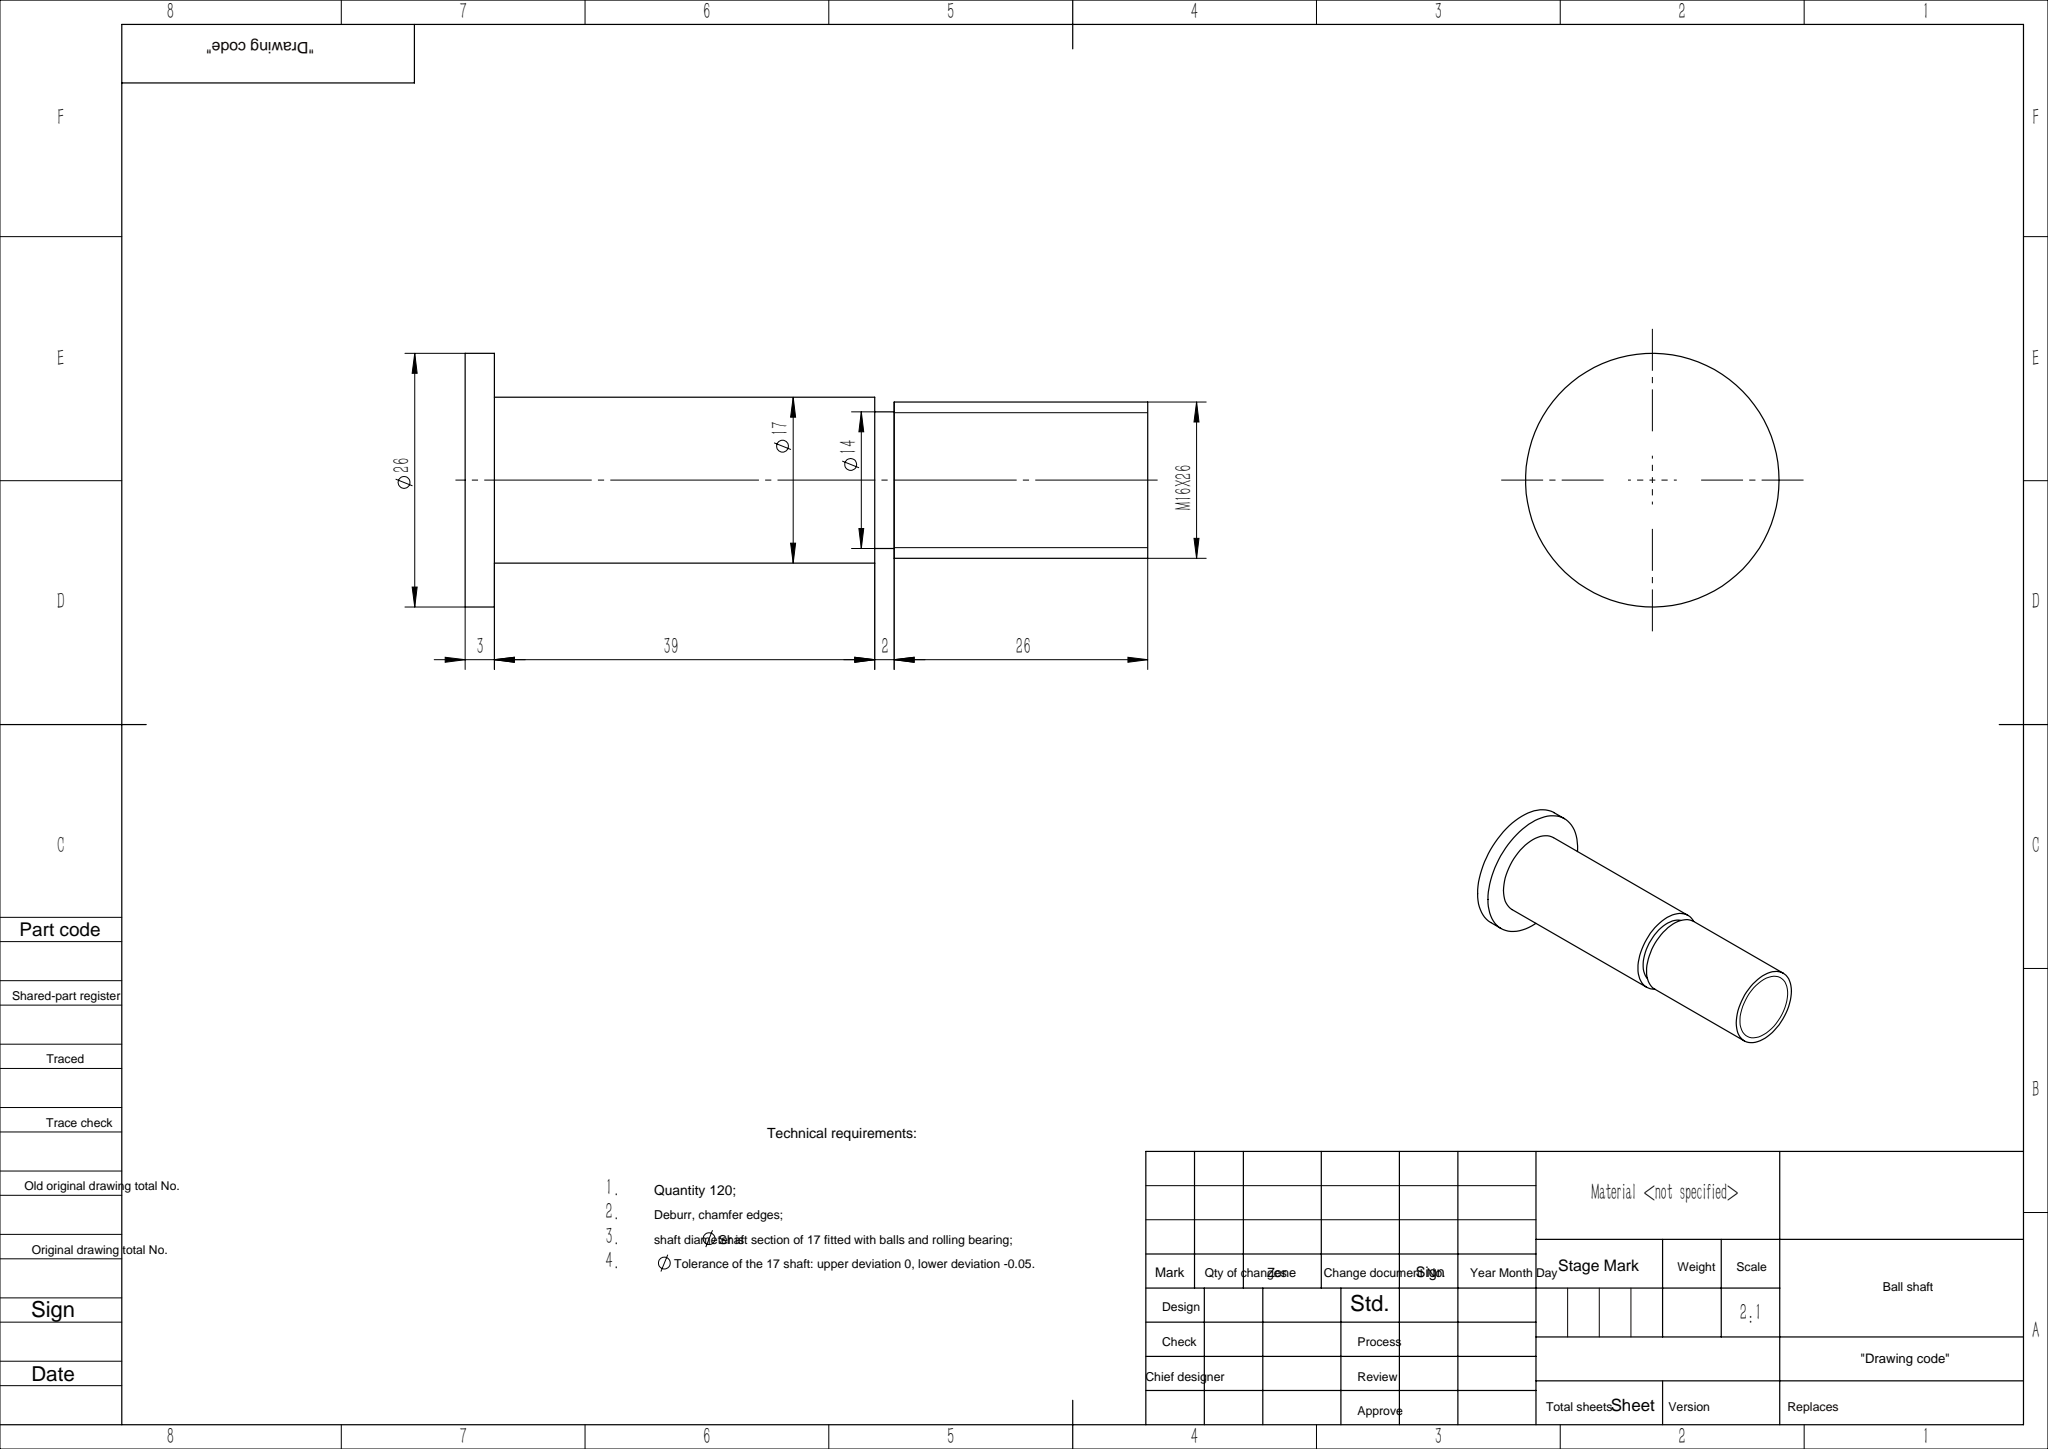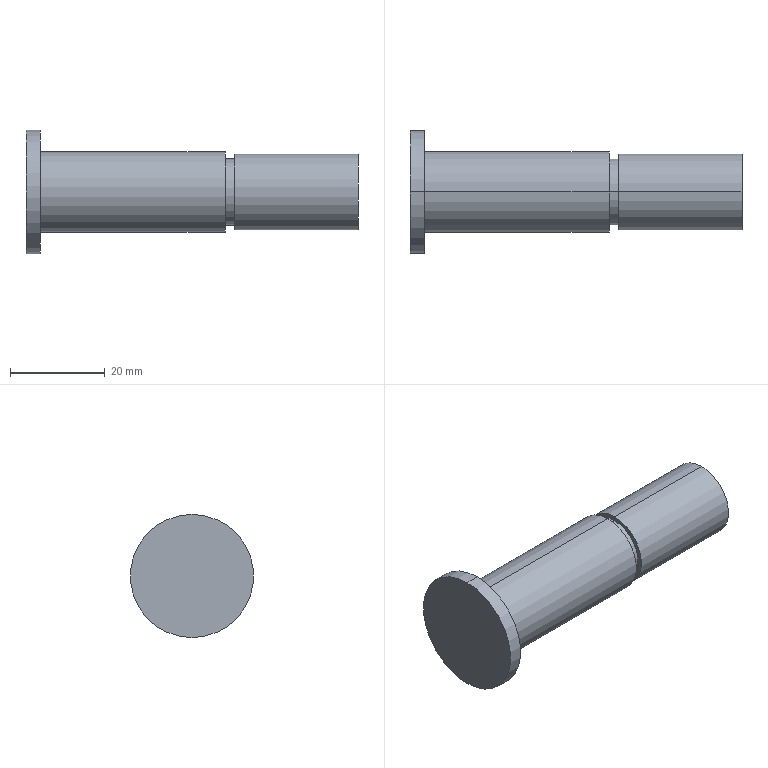Part | SolidWorks | features ICE 2, Revolution 1 | 1 solid | 13 faces | box 70 x 26 x 26 mm | volume 15980 mm3 | cylinder 8 | plane 5 | commonest cylinder face diameters 14 x2 16 x2 17 x2 26 x2
STEP:
#1=CARTESIAN_POINT('',(44.,0.,-8.));
#2=VERTEX_POINT('',#1);
#3=CARTESIAN_POINT('',(44.,0.,8.));
#4=VERTEX_POINT('',#3);
#5=CARTESIAN_POINT('',(44.,0.,0.));
#6=DIRECTION('',(1.,0.,0.));
#7=DIRECTION('',(0.,0.,-1.));
#8=AXIS2_PLACEMENT_3D('',#5,#6,#7);
#9=CIRCLE('',#8,8.);
#10=EDGE_CURVE('',#2,#4,#9,.T.);
#11=ORIENTED_EDGE('',*,*,#10,.T.);
#12=CARTESIAN_POINT('',(70.,0.,8.));
#13=VERTEX_POINT('',#12);
#14=CARTESIAN_POINT('',(42.,0.,8.));
#15=DIRECTION('',(1.,0.,0.));
#16=VECTOR('',#15,1000.);
#17=LINE('',#14,#16);
#18=EDGE_CURVE('',#4,#13,#17,.T.);
#19=ORIENTED_EDGE('',*,*,#18,.T.);
#20=CARTESIAN_POINT('',(70.,0.,-8.));
#21=VERTEX_POINT('',#20);
#22=CARTESIAN_POINT('',(70.,0.,0.));
#23=DIRECTION('',(1.,0.,0.));
#24=DIRECTION('',(0.,0.,-1.));
#25=AXIS2_PLACEMENT_3D('',#22,#23,#24);
#26=CIRCLE('',#25,8.);
#27=EDGE_CURVE('',#21,#13,#26,.T.);
#28=ORIENTED_EDGE('',*,*,#27,.F.);
#29=CARTESIAN_POINT('',(42.,0.,-8.));
#30=DIRECTION('',(1.,0.,0.));
#31=VECTOR('',#30,1000.);
#32=LINE('',#29,#31);
#33=EDGE_CURVE('',#2,#21,#32,.T.);
#34=ORIENTED_EDGE('',*,*,#33,.F.);
#35=EDGE_LOOP('',(#11,#19,#28,#34));
#36=FACE_OUTER_BOUND('',#35,.T.);
#37=CARTESIAN_POINT('',(42.,0.,0.));
#38=DIRECTION('',(1.,0.,0.));
#39=DIRECTION('',(0.,0.,-1.));
#40=AXIS2_PLACEMENT_3D('',#37,#38,#39);
#41=CYLINDRICAL_SURFACE('',#40,8.);
#42=ADVANCED_FACE('',(#36),#41,.T.);
#43=CARTESIAN_POINT('',(44.,0.,-7.));
#44=VERTEX_POINT('',#43);
#45=CARTESIAN_POINT('',(44.,0.,7.));
#46=VERTEX_POINT('',#45);
#47=CARTESIAN_POINT('',(44.,0.,0.));
#48=DIRECTION('',(1.,0.,0.));
#49=DIRECTION('',(0.,0.,-1.));
#50=AXIS2_PLACEMENT_3D('',#47,#48,#49);
#51=CIRCLE('',#50,7.);
#52=EDGE_CURVE('',#44,#46,#51,.T.);
#53=ORIENTED_EDGE('',*,*,#52,.F.);
#54=CARTESIAN_POINT('',(42.,0.,-7.));
#55=VERTEX_POINT('',#54);
#56=CARTESIAN_POINT('',(44.,0.,-7.));
#57=DIRECTION('',(-1.,0.,0.));
#58=VECTOR('',#57,1000.);
#59=LINE('',#56,#58);
#60=EDGE_CURVE('',#44,#55,#59,.T.);
#61=ORIENTED_EDGE('',*,*,#60,.T.);
#62=CARTESIAN_POINT('',(42.,0.,7.));
#63=VERTEX_POINT('',#62);
#64=CARTESIAN_POINT('',(42.,0.,0.));
#65=DIRECTION('',(1.,0.,0.));
#66=DIRECTION('',(0.,0.,-1.));
#67=AXIS2_PLACEMENT_3D('',#64,#65,#66);
#68=CIRCLE('',#67,7.);
#69=EDGE_CURVE('',#55,#63,#68,.T.);
#70=ORIENTED_EDGE('',*,*,#69,.T.);
#71=CARTESIAN_POINT('',(44.,0.,7.));
#72=DIRECTION('',(-1.,0.,0.));
#73=VECTOR('',#72,1000.);
#74=LINE('',#71,#73);
#75=EDGE_CURVE('',#46,#63,#74,.T.);
#76=ORIENTED_EDGE('',*,*,#75,.F.);
#77=EDGE_LOOP('',(#53,#61,#70,#76));
#78=FACE_OUTER_BOUND('',#77,.T.);
#79=CARTESIAN_POINT('',(44.,0.,0.));
#80=DIRECTION('',(-1.,0.,0.));
#81=DIRECTION('',(0.,0.,1.));
#82=AXIS2_PLACEMENT_3D('',#79,#80,#81);
#83=CYLINDRICAL_SURFACE('',#82,7.);
#84=ADVANCED_FACE('',(#78),#83,.T.);
#85=CARTESIAN_POINT('',(3.,0.,13.));
#86=VERTEX_POINT('',#85);
#87=CARTESIAN_POINT('',(3.,0.,-13.));
#88=VERTEX_POINT('',#87);
#89=CARTESIAN_POINT('',(3.,0.,0.));
#90=DIRECTION('',(-1.,0.,0.));
#91=DIRECTION('',(0.,0.,1.));
#92=AXIS2_PLACEMENT_3D('',#89,#90,#91);
#93=CIRCLE('',#92,13.);
#94=EDGE_CURVE('',#86,#88,#93,.T.);
#95=ORIENTED_EDGE('',*,*,#94,.T.);
#96=CARTESIAN_POINT('',(0.,0.,-13.));
#97=VERTEX_POINT('',#96);
#98=CARTESIAN_POINT('',(0.,0.,-13.));
#99=DIRECTION('',(-1.,0.,0.));
#100=VECTOR('',#99,1000.);
#101=LINE('',#98,#100);
#102=EDGE_CURVE('',#88,#97,#101,.T.);
#103=ORIENTED_EDGE('',*,*,#102,.T.);
#104=CARTESIAN_POINT('',(0.,0.,13.));
#105=VERTEX_POINT('',#104);
#106=CARTESIAN_POINT('',(0.,0.,0.));
#107=DIRECTION('',(-1.,0.,0.));
#108=DIRECTION('',(0.,0.,1.));
#109=AXIS2_PLACEMENT_3D('',#106,#107,#108);
#110=CIRCLE('',#109,13.);
#111=EDGE_CURVE('',#105,#97,#110,.T.);
#112=ORIENTED_EDGE('',*,*,#111,.F.);
#113=CARTESIAN_POINT('',(0.,0.,13.));
#114=DIRECTION('',(-1.,0.,0.));
#115=VECTOR('',#114,1000.);
#116=LINE('',#113,#115);
#117=EDGE_CURVE('',#86,#105,#116,.T.);
#118=ORIENTED_EDGE('',*,*,#117,.F.);
#119=EDGE_LOOP('',(#95,#103,#112,#118));
#120=FACE_OUTER_BOUND('',#119,.T.);
#121=CARTESIAN_POINT('',(0.,0.,0.));
#122=DIRECTION('',(-1.,0.,0.));
#123=DIRECTION('',(0.,0.,1.));
#124=AXIS2_PLACEMENT_3D('',#121,#122,#123);
#125=CYLINDRICAL_SURFACE('',#124,13.);
#126=ADVANCED_FACE('',(#120),#125,.T.);
#127=CARTESIAN_POINT('',(42.,0.,-8.5));
#128=VERTEX_POINT('',#127);
#129=CARTESIAN_POINT('',(42.,0.,8.5));
#130=VERTEX_POINT('',#129);
#131=CARTESIAN_POINT('',(42.,0.,0.));
#132=DIRECTION('',(1.,0.,0.));
#133=DIRECTION('',(0.,0.,-1.));
#134=AXIS2_PLACEMENT_3D('',#131,#132,#133);
#135=CIRCLE('',#134,8.5);
#136=EDGE_CURVE('',#128,#130,#135,.T.);
#137=ORIENTED_EDGE('',*,*,#136,.F.);
#138=CARTESIAN_POINT('',(3.,0.,-8.5));
#139=VERTEX_POINT('',#138);
#140=CARTESIAN_POINT('',(0.,0.,-8.5));
#141=DIRECTION('',(-1.,0.,0.));
#142=VECTOR('',#141,1000.);
#143=LINE('',#140,#142);
#144=EDGE_CURVE('',#128,#139,#143,.T.);
#145=ORIENTED_EDGE('',*,*,#144,.T.);
#146=CARTESIAN_POINT('',(3.,0.,8.5));
#147=VERTEX_POINT('',#146);
#148=CARTESIAN_POINT('',(3.,0.,0.));
#149=DIRECTION('',(-1.,0.,0.));
#150=DIRECTION('',(0.,0.,1.));
#151=AXIS2_PLACEMENT_3D('',#148,#149,#150);
#152=CIRCLE('',#151,8.5);
#153=EDGE_CURVE('',#147,#139,#152,.T.);
#154=ORIENTED_EDGE('',*,*,#153,.F.);
#155=CARTESIAN_POINT('',(0.,0.,8.5));
#156=DIRECTION('',(-1.,0.,0.));
#157=VECTOR('',#156,1000.);
#158=LINE('',#155,#157);
#159=EDGE_CURVE('',#130,#147,#158,.T.);
#160=ORIENTED_EDGE('',*,*,#159,.F.);
#161=EDGE_LOOP('',(#137,#145,#154,#160));
#162=FACE_OUTER_BOUND('',#161,.T.);
#163=CARTESIAN_POINT('',(0.,0.,0.));
#164=DIRECTION('',(-1.,0.,0.));
#165=DIRECTION('',(0.,0.,1.));
#166=AXIS2_PLACEMENT_3D('',#163,#164,#165);
#167=CYLINDRICAL_SURFACE('',#166,8.5);
#168=ADVANCED_FACE('',(#162),#167,.T.);
#169=ORIENTED_EDGE('',*,*,#144,.F.);
#170=CARTESIAN_POINT('',(42.,0.,0.));
#171=DIRECTION('',(1.,0.,0.));
#172=DIRECTION('',(0.,0.,-1.));
#173=AXIS2_PLACEMENT_3D('',#170,#171,#172);
#174=CIRCLE('',#173,8.5);
#175=EDGE_CURVE('',#130,#128,#174,.T.);
#176=ORIENTED_EDGE('',*,*,#175,.F.);
#177=ORIENTED_EDGE('',*,*,#159,.T.);
#178=CARTESIAN_POINT('',(3.,0.,0.));
#179=DIRECTION('',(-1.,0.,0.));
#180=DIRECTION('',(0.,0.,1.));
#181=AXIS2_PLACEMENT_3D('',#178,#179,#180);
#182=CIRCLE('',#181,8.5);
#183=EDGE_CURVE('',#139,#147,#182,.T.);
#184=ORIENTED_EDGE('',*,*,#183,.F.);
#185=EDGE_LOOP('',(#169,#176,#177,#184));
#186=FACE_OUTER_BOUND('',#185,.T.);
#187=CARTESIAN_POINT('',(0.,0.,0.));
#188=DIRECTION('',(-1.,0.,0.));
#189=DIRECTION('',(0.,0.,1.));
#190=AXIS2_PLACEMENT_3D('',#187,#188,#189);
#191=CYLINDRICAL_SURFACE('',#190,8.5);
#192=ADVANCED_FACE('',(#186),#191,.T.);
#193=ORIENTED_EDGE('',*,*,#111,.T.);
#194=CARTESIAN_POINT('',(0.,0.,0.));
#195=DIRECTION('',(-1.,0.,0.));
#196=DIRECTION('',(0.,0.,1.));
#197=AXIS2_PLACEMENT_3D('',#194,#195,#196);
#198=CIRCLE('',#197,13.);
#199=EDGE_CURVE('',#97,#105,#198,.T.);
#200=ORIENTED_EDGE('',*,*,#199,.T.);
#201=EDGE_LOOP('',(#193,#200));
#202=FACE_OUTER_BOUND('',#201,.T.);
#203=CARTESIAN_POINT('',(0.,0.,0.));
#204=DIRECTION('',(1.,0.,0.));
#205=DIRECTION('',(0.,0.,-1.));
#206=AXIS2_PLACEMENT_3D('',#203,#204,#205);
#207=PLANE('',#206);
#208=ADVANCED_FACE('',(#202),#207,.F.);
#209=ORIENTED_EDGE('',*,*,#102,.F.);
#210=CARTESIAN_POINT('',(3.,0.,0.));
#211=DIRECTION('',(-1.,0.,0.));
#212=DIRECTION('',(0.,0.,1.));
#213=AXIS2_PLACEMENT_3D('',#210,#211,#212);
#214=CIRCLE('',#213,13.);
#215=EDGE_CURVE('',#88,#86,#214,.T.);
#216=ORIENTED_EDGE('',*,*,#215,.T.);
#217=ORIENTED_EDGE('',*,*,#117,.T.);
#218=ORIENTED_EDGE('',*,*,#199,.F.);
#219=EDGE_LOOP('',(#209,#216,#217,#218));
#220=FACE_OUTER_BOUND('',#219,.T.);
#221=CARTESIAN_POINT('',(0.,0.,0.));
#222=DIRECTION('',(-1.,0.,0.));
#223=DIRECTION('',(0.,0.,1.));
#224=AXIS2_PLACEMENT_3D('',#221,#222,#223);
#225=CYLINDRICAL_SURFACE('',#224,13.);
#226=ADVANCED_FACE('',(#220),#225,.T.);
#227=ORIENTED_EDGE('',*,*,#94,.F.);
#228=ORIENTED_EDGE('',*,*,#215,.F.);
#229=EDGE_LOOP('',(#227,#228));
#230=FACE_OUTER_BOUND('',#229,.T.);
#231=ORIENTED_EDGE('',*,*,#153,.T.);
#232=ORIENTED_EDGE('',*,*,#183,.T.);
#233=EDGE_LOOP('',(#231,#232));
#234=FACE_BOUND('',#233,.T.);
#235=CARTESIAN_POINT('',(3.,13.,0.));
#236=DIRECTION('',(-1.,0.,0.));
#237=DIRECTION('',(0.,0.,1.));
#238=AXIS2_PLACEMENT_3D('',#235,#236,#237);
#239=PLANE('',#238);
#240=ADVANCED_FACE('',(#230,#234),#239,.F.);
#241=ORIENTED_EDGE('',*,*,#175,.T.);
#242=ORIENTED_EDGE('',*,*,#136,.T.);
#243=EDGE_LOOP('',(#241,#242));
#244=FACE_OUTER_BOUND('',#243,.T.);
#245=CARTESIAN_POINT('',(42.,0.,0.));
#246=DIRECTION('',(1.,0.,0.));
#247=DIRECTION('',(0.,0.,-1.));
#248=AXIS2_PLACEMENT_3D('',#245,#246,#247);
#249=CIRCLE('',#248,7.);
#250=EDGE_CURVE('',#63,#55,#249,.T.);
#251=ORIENTED_EDGE('',*,*,#250,.F.);
#252=ORIENTED_EDGE('',*,*,#69,.F.);
#253=EDGE_LOOP('',(#251,#252));
#254=FACE_BOUND('',#253,.T.);
#255=CARTESIAN_POINT('',(42.,0.,0.));
#256=DIRECTION('',(1.,0.,0.));
#257=DIRECTION('',(0.,0.,-1.));
#258=AXIS2_PLACEMENT_3D('',#255,#256,#257);
#259=PLANE('',#258);
#260=ADVANCED_FACE('',(#244,#254),#259,.T.);
#261=ORIENTED_EDGE('',*,*,#10,.F.);
#262=CARTESIAN_POINT('',(44.,0.,0.));
#263=DIRECTION('',(1.,0.,0.));
#264=DIRECTION('',(0.,0.,-1.));
#265=AXIS2_PLACEMENT_3D('',#262,#263,#264);
#266=CIRCLE('',#265,8.);
#267=EDGE_CURVE('',#4,#2,#266,.T.);
#268=ORIENTED_EDGE('',*,*,#267,.F.);
#269=EDGE_LOOP('',(#261,#268));
#270=FACE_OUTER_BOUND('',#269,.T.);
#271=CARTESIAN_POINT('',(44.,0.,0.));
#272=DIRECTION('',(1.,0.,0.));
#273=DIRECTION('',(0.,0.,-1.));
#274=AXIS2_PLACEMENT_3D('',#271,#272,#273);
#275=CIRCLE('',#274,7.);
#276=EDGE_CURVE('',#46,#44,#275,.T.);
#277=ORIENTED_EDGE('',*,*,#276,.T.);
#278=ORIENTED_EDGE('',*,*,#52,.T.);
#279=EDGE_LOOP('',(#277,#278));
#280=FACE_BOUND('',#279,.T.);
#281=CARTESIAN_POINT('',(44.,0.,0.));
#282=DIRECTION('',(1.,0.,0.));
#283=DIRECTION('',(0.,0.,-1.));
#284=AXIS2_PLACEMENT_3D('',#281,#282,#283);
#285=PLANE('',#284);
#286=ADVANCED_FACE('',(#270,#280),#285,.F.);
#287=ORIENTED_EDGE('',*,*,#60,.F.);
#288=ORIENTED_EDGE('',*,*,#276,.F.);
#289=ORIENTED_EDGE('',*,*,#75,.T.);
#290=ORIENTED_EDGE('',*,*,#250,.T.);
#291=EDGE_LOOP('',(#287,#288,#289,#290));
#292=FACE_OUTER_BOUND('',#291,.T.);
#293=CARTESIAN_POINT('',(44.,0.,0.));
#294=DIRECTION('',(-1.,0.,0.));
#295=DIRECTION('',(0.,0.,1.));
#296=AXIS2_PLACEMENT_3D('',#293,#294,#295);
#297=CYLINDRICAL_SURFACE('',#296,7.);
#298=ADVANCED_FACE('',(#292),#297,.T.);
#299=ORIENTED_EDGE('',*,*,#27,.T.);
#300=CARTESIAN_POINT('',(70.,0.,0.));
#301=DIRECTION('',(1.,0.,0.));
#302=DIRECTION('',(0.,0.,-1.));
#303=AXIS2_PLACEMENT_3D('',#300,#301,#302);
#304=CIRCLE('',#303,8.);
#305=EDGE_CURVE('',#13,#21,#304,.T.);
#306=ORIENTED_EDGE('',*,*,#305,.T.);
#307=EDGE_LOOP('',(#299,#306));
#308=FACE_OUTER_BOUND('',#307,.T.);
#309=CARTESIAN_POINT('',(70.,8.5,0.));
#310=DIRECTION('',(-1.,0.,0.));
#311=DIRECTION('',(0.,0.,1.));
#312=AXIS2_PLACEMENT_3D('',#309,#310,#311);
#313=PLANE('',#312);
#314=ADVANCED_FACE('',(#308),#313,.F.);
#315=ORIENTED_EDGE('',*,*,#18,.F.);
#316=ORIENTED_EDGE('',*,*,#267,.T.);
#317=ORIENTED_EDGE('',*,*,#33,.T.);
#318=ORIENTED_EDGE('',*,*,#305,.F.);
#319=EDGE_LOOP('',(#315,#316,#317,#318));
#320=FACE_OUTER_BOUND('',#319,.T.);
#321=CARTESIAN_POINT('',(42.,0.,0.));
#322=DIRECTION('',(1.,0.,0.));
#323=DIRECTION('',(0.,0.,-1.));
#324=AXIS2_PLACEMENT_3D('',#321,#322,#323);
#325=CYLINDRICAL_SURFACE('',#324,8.);
#326=ADVANCED_FACE('',(#320),#325,.T.);
#327=CLOSED_SHELL('',(#42,#84,#126,#168,#192,#208,#226,#240,#260,#286,#298,#314,#326));
#328=MANIFOLD_SOLID_BREP('',#327);
#329=CARTESIAN_POINT('',(0.,0.,0.));
#330=DIRECTION('',(0.,0.,1.));
#331=DIRECTION('',(1.,0.,0.));
#332=AXIS2_PLACEMENT_3D('',#329,#330,#331);
#333=(LENGTH_UNIT()NAMED_UNIT(*)SI_UNIT(.MILLI.,.METRE.));
#334=UNCERTAINTY_MEASURE_WITH_UNIT(LENGTH_MEASURE(0.00001),#333,'','');
#335=(NAMED_UNIT(*)PLANE_ANGLE_UNIT()SI_UNIT($,.RADIAN.));
#336=(NAMED_UNIT(*)SI_UNIT($,.STERADIAN.)SOLID_ANGLE_UNIT());
#337=(GEOMETRIC_REPRESENTATION_CONTEXT(3)GLOBAL_UNCERTAINTY_ASSIGNED_CONTEXT((#334))GLOBAL_UNIT_ASSIGNED_CONTEXT((#333,#335,#336))REPRESENTATION_CONTEXT('',''));
#338=ADVANCED_BREP_SHAPE_REPRESENTATION('',(#328,#332),#337);